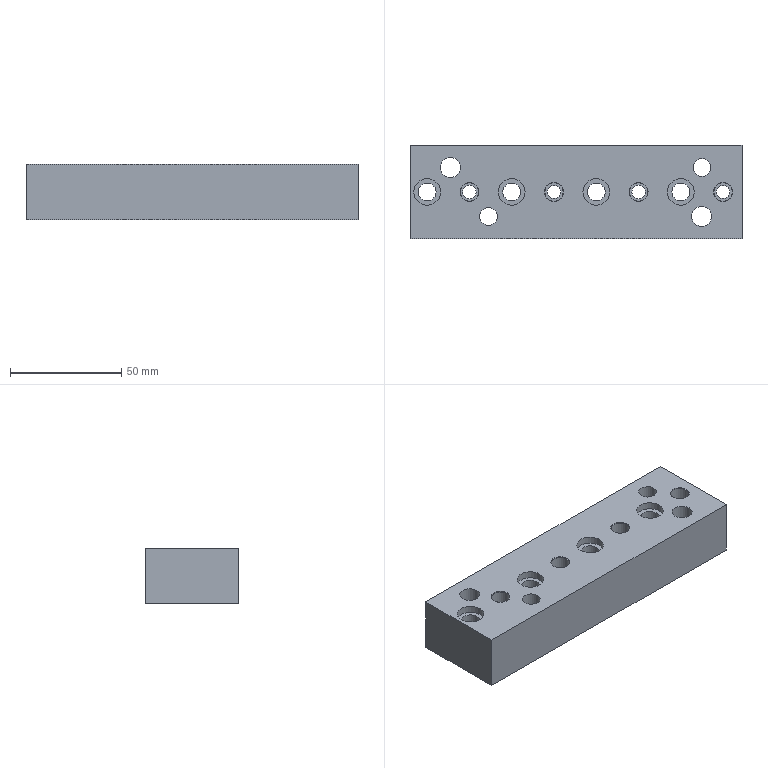Part | STEP file | PN_0036_id230_x_t | 1 solid | 46 faces | box 149.23 x 42 x 25 mm | volume 138214 mm3 | cylinder 26 | plane 20 | commonest cylinder face diameters 8 x6 6 x4 8.2 x4 8.5 x4 12 x4 9 x2
STEP:
#1=CARTESIAN_POINT('',(87.422,21.,25.));
#2=VERTEX_POINT('',#1);
#3=CARTESIAN_POINT('',(236.5,21.,25.));
#4=VERTEX_POINT('',#3);
#5=CARTESIAN_POINT('',(27.5,21.,25.));
#6=DIRECTION('',(1.,0.,0.));
#7=VECTOR('',#6,1.);
#8=LINE('',#5,#7);
#9=EDGE_CURVE('',#2,#4,#8,.T.);
#10=ORIENTED_EDGE('',*,*,#9,.T.);
#11=CARTESIAN_POINT('',(236.5,21.,0.));
#12=VERTEX_POINT('',#11);
#13=CARTESIAN_POINT('',(236.5,21.,12.5));
#14=DIRECTION('',(0.,0.,1.));
#15=VECTOR('',#14,1.);
#16=LINE('',#13,#15);
#17=EDGE_CURVE('',#12,#4,#16,.T.);
#18=ORIENTED_EDGE('',*,*,#17,.F.);
#19=CARTESIAN_POINT('',(87.422,21.,0.));
#20=VERTEX_POINT('',#19);
#21=CARTESIAN_POINT('',(27.5,21.,0.));
#22=DIRECTION('',(-1.,0.,0.));
#23=VECTOR('',#22,1.);
#24=LINE('',#21,#23);
#25=EDGE_CURVE('',#12,#20,#24,.T.);
#26=ORIENTED_EDGE('',*,*,#25,.T.);
#27=CARTESIAN_POINT('',(87.422,21.,12.5));
#28=DIRECTION('',(0.,0.,1.));
#29=VECTOR('',#28,1.);
#30=LINE('',#27,#29);
#31=EDGE_CURVE('',#20,#2,#30,.T.);
#32=ORIENTED_EDGE('',*,*,#31,.T.);
#33=EDGE_LOOP('',(#10,#18,#26,#32));
#34=FACE_OUTER_BOUND('',#33,.T.);
#35=CARTESIAN_POINT('',(47.5,21.,12.5));
#36=DIRECTION('',(0.,1.,0.));
#37=DIRECTION('',(0.,0.,1.));
#38=AXIS2_PLACEMENT_3D('',#35,#36,#37);
#39=PLANE('',#38);
#40=ADVANCED_FACE('',(#34),#39,.T.);
#41=CARTESIAN_POINT('',(87.27,-21.,0.));
#42=VERTEX_POINT('',#41);
#43=CARTESIAN_POINT('',(236.5,-21.,0.));
#44=VERTEX_POINT('',#43);
#45=CARTESIAN_POINT('',(27.5,-21.,0.));
#46=DIRECTION('',(1.,0.,0.));
#47=VECTOR('',#46,1.);
#48=LINE('',#45,#47);
#49=EDGE_CURVE('',#42,#44,#48,.T.);
#50=ORIENTED_EDGE('',*,*,#49,.T.);
#51=CARTESIAN_POINT('',(236.5,-21.,25.));
#52=VERTEX_POINT('',#51);
#53=CARTESIAN_POINT('',(236.5,-21.,12.5));
#54=DIRECTION('',(0.,0.,1.));
#55=VECTOR('',#54,1.);
#56=LINE('',#53,#55);
#57=EDGE_CURVE('',#44,#52,#56,.T.);
#58=ORIENTED_EDGE('',*,*,#57,.T.);
#59=CARTESIAN_POINT('',(87.27,-21.,25.));
#60=VERTEX_POINT('',#59);
#61=CARTESIAN_POINT('',(27.5,-21.,25.));
#62=DIRECTION('',(-1.,0.,0.));
#63=VECTOR('',#62,1.);
#64=LINE('',#61,#63);
#65=EDGE_CURVE('',#52,#60,#64,.T.);
#66=ORIENTED_EDGE('',*,*,#65,.T.);
#67=CARTESIAN_POINT('',(87.27,-21.,25.818));
#68=DIRECTION('',(0.,0.,1.));
#69=VECTOR('',#68,1.);
#70=LINE('',#67,#69);
#71=EDGE_CURVE('',#42,#60,#70,.T.);
#72=ORIENTED_EDGE('',*,*,#71,.F.);
#73=EDGE_LOOP('',(#50,#58,#66,#72));
#74=FACE_OUTER_BOUND('',#73,.T.);
#75=CARTESIAN_POINT('',(110.347,-21.,25.818));
#76=DIRECTION('',(0.,1.,0.));
#77=DIRECTION('',(0.,0.,1.));
#78=AXIS2_PLACEMENT_3D('',#75,#76,#77);
#79=PLANE('',#78);
#80=ADVANCED_FACE('',(#74),#79,.F.);
#81=CARTESIAN_POINT('',(118.5,-11.,25.));
#82=VERTEX_POINT('',#81);
#83=CARTESIAN_POINT('',(122.5,-11.,25.));
#84=DIRECTION('',(0.,0.,-1.));
#85=DIRECTION('',(-1.,0.,0.));
#86=AXIS2_PLACEMENT_3D('',#83,#84,#85);
#87=CIRCLE('',#86,4.);
#88=EDGE_CURVE('',#82,#82,#87,.T.);
#89=ORIENTED_EDGE('',*,*,#88,.T.);
#90=EDGE_LOOP('',(#89));
#91=FACE_BOUND('',#90,.T.);
#92=CARTESIAN_POINT('',(214.5,11.,25.));
#93=VERTEX_POINT('',#92);
#94=CARTESIAN_POINT('',(218.5,11.,25.));
#95=DIRECTION('',(0.,0.,-1.));
#96=DIRECTION('',(-1.,0.,0.));
#97=AXIS2_PLACEMENT_3D('',#94,#95,#96);
#98=CIRCLE('',#97,4.);
#99=EDGE_CURVE('',#93,#93,#98,.T.);
#100=ORIENTED_EDGE('',*,*,#99,.T.);
#101=EDGE_LOOP('',(#100));
#102=FACE_BOUND('',#101,.T.);
#103=CARTESIAN_POINT('',(222.848,-11.,25.));
#104=VERTEX_POINT('',#103);
#105=CARTESIAN_POINT('',(218.348,-11.,25.));
#106=DIRECTION('',(0.,0.,-1.));
#107=DIRECTION('',(1.,0.,0.));
#108=AXIS2_PLACEMENT_3D('',#105,#106,#107);
#109=CIRCLE('',#108,4.5);
#110=EDGE_CURVE('',#104,#104,#109,.T.);
#111=ORIENTED_EDGE('',*,*,#110,.T.);
#112=EDGE_LOOP('',(#111));
#113=FACE_BOUND('',#112,.T.);
#114=CARTESIAN_POINT('',(100.922,11.,25.));
#115=VERTEX_POINT('',#114);
#116=CARTESIAN_POINT('',(105.422,11.,25.));
#117=DIRECTION('',(0.,0.,-1.));
#118=DIRECTION('',(-1.,0.,0.));
#119=AXIS2_PLACEMENT_3D('',#116,#117,#118);
#120=CIRCLE('',#119,4.5);
#121=EDGE_CURVE('',#115,#115,#120,.T.);
#122=ORIENTED_EDGE('',*,*,#121,.T.);
#123=EDGE_LOOP('',(#122));
#124=FACE_BOUND('',#123,.T.);
#125=CARTESIAN_POINT('',(232.25,0.,25.));
#126=VERTEX_POINT('',#125);
#127=CARTESIAN_POINT('',(228.,0.,25.));
#128=DIRECTION('',(0.,0.,1.));
#129=DIRECTION('',(1.,0.,0.));
#130=AXIS2_PLACEMENT_3D('',#127,#128,#129);
#131=CIRCLE('',#130,4.25);
#132=EDGE_CURVE('',#126,#126,#131,.T.);
#133=ORIENTED_EDGE('',*,*,#132,.F.);
#134=EDGE_LOOP('',(#133));
#135=FACE_BOUND('',#134,.T.);
#136=CARTESIAN_POINT('',(194.25,0.,25.));
#137=VERTEX_POINT('',#136);
#138=CARTESIAN_POINT('',(190.,0.,25.));
#139=DIRECTION('',(0.,0.,1.));
#140=DIRECTION('',(1.,0.,0.));
#141=AXIS2_PLACEMENT_3D('',#138,#139,#140);
#142=CIRCLE('',#141,4.25);
#143=EDGE_CURVE('',#137,#137,#142,.T.);
#144=ORIENTED_EDGE('',*,*,#143,.F.);
#145=EDGE_LOOP('',(#144));
#146=FACE_BOUND('',#145,.T.);
#147=CARTESIAN_POINT('',(156.25,0.,25.));
#148=VERTEX_POINT('',#147);
#149=CARTESIAN_POINT('',(152.,0.,25.));
#150=DIRECTION('',(0.,0.,1.));
#151=DIRECTION('',(1.,0.,0.));
#152=AXIS2_PLACEMENT_3D('',#149,#150,#151);
#153=CIRCLE('',#152,4.25);
#154=EDGE_CURVE('',#148,#148,#153,.T.);
#155=ORIENTED_EDGE('',*,*,#154,.F.);
#156=EDGE_LOOP('',(#155));
#157=FACE_BOUND('',#156,.T.);
#158=CARTESIAN_POINT('',(118.25,0.,25.));
#159=VERTEX_POINT('',#158);
#160=CARTESIAN_POINT('',(114.,0.,25.));
#161=DIRECTION('',(0.,0.,1.));
#162=DIRECTION('',(1.,0.,0.));
#163=AXIS2_PLACEMENT_3D('',#160,#161,#162);
#164=CIRCLE('',#163,4.25);
#165=EDGE_CURVE('',#159,#159,#164,.T.);
#166=ORIENTED_EDGE('',*,*,#165,.F.);
#167=EDGE_LOOP('',(#166));
#168=FACE_BOUND('',#167,.T.);
#169=CARTESIAN_POINT('',(215.,0.,25.));
#170=VERTEX_POINT('',#169);
#171=CARTESIAN_POINT('',(209.,0.,25.));
#172=DIRECTION('',(0.,0.,-1.));
#173=DIRECTION('',(1.,0.,0.));
#174=AXIS2_PLACEMENT_3D('',#171,#172,#173);
#175=CIRCLE('',#174,6.);
#176=EDGE_CURVE('',#170,#170,#175,.T.);
#177=ORIENTED_EDGE('',*,*,#176,.T.);
#178=EDGE_LOOP('',(#177));
#179=FACE_BOUND('',#178,.T.);
#180=CARTESIAN_POINT('',(177.,0.,25.));
#181=VERTEX_POINT('',#180);
#182=CARTESIAN_POINT('',(171.,0.,25.));
#183=DIRECTION('',(0.,0.,-1.));
#184=DIRECTION('',(1.,0.,0.));
#185=AXIS2_PLACEMENT_3D('',#182,#183,#184);
#186=CIRCLE('',#185,6.);
#187=EDGE_CURVE('',#181,#181,#186,.T.);
#188=ORIENTED_EDGE('',*,*,#187,.T.);
#189=EDGE_LOOP('',(#188));
#190=FACE_BOUND('',#189,.T.);
#191=CARTESIAN_POINT('',(139.,0.,25.));
#192=VERTEX_POINT('',#191);
#193=CARTESIAN_POINT('',(133.,0.,25.));
#194=DIRECTION('',(0.,0.,-1.));
#195=DIRECTION('',(1.,0.,0.));
#196=AXIS2_PLACEMENT_3D('',#193,#194,#195);
#197=CIRCLE('',#196,6.);
#198=EDGE_CURVE('',#192,#192,#197,.T.);
#199=ORIENTED_EDGE('',*,*,#198,.T.);
#200=EDGE_LOOP('',(#199));
#201=FACE_BOUND('',#200,.T.);
#202=CARTESIAN_POINT('',(101.,0.,25.));
#203=VERTEX_POINT('',#202);
#204=CARTESIAN_POINT('',(95.,0.,25.));
#205=DIRECTION('',(0.,0.,-1.));
#206=DIRECTION('',(1.,0.,0.));
#207=AXIS2_PLACEMENT_3D('',#204,#205,#206);
#208=CIRCLE('',#207,6.);
#209=EDGE_CURVE('',#203,#203,#208,.T.);
#210=ORIENTED_EDGE('',*,*,#209,.T.);
#211=EDGE_LOOP('',(#210));
#212=FACE_BOUND('',#211,.T.);
#213=ORIENTED_EDGE('',*,*,#65,.F.);
#214=CARTESIAN_POINT('',(236.5,-7.4,25.));
#215=DIRECTION('',(0.,-1.,0.));
#216=VECTOR('',#215,1.);
#217=LINE('',#214,#216);
#218=EDGE_CURVE('',#4,#52,#217,.T.);
#219=ORIENTED_EDGE('',*,*,#218,.F.);
#220=ORIENTED_EDGE('',*,*,#9,.F.);
#221=CARTESIAN_POINT('',(87.319,-7.617,25.));
#222=DIRECTION('',(-0.003625,-1.,0.));
#223=VECTOR('',#222,1.);
#224=LINE('',#221,#223);
#225=EDGE_CURVE('',#2,#60,#224,.T.);
#226=ORIENTED_EDGE('',*,*,#225,.T.);
#227=EDGE_LOOP('',(#213,#219,#220,#226));
#228=FACE_BOUND('',#227,.T.);
#229=CARTESIAN_POINT('',(27.5,-7.4,25.));
#230=DIRECTION('',(0.,0.,1.));
#231=DIRECTION('',(0.,-1.,0.));
#232=AXIS2_PLACEMENT_3D('',#229,#230,#231);
#233=PLANE('',#232);
#234=ADVANCED_FACE('',(#91,#102,#113,#124,#135,#146,#157,#168,#179,#190,#201,#212,#228),#233,.T.);
#235=CARTESIAN_POINT('',(118.5,-11.,0.));
#236=VERTEX_POINT('',#235);
#237=CARTESIAN_POINT('',(122.5,-11.,0.));
#238=DIRECTION('',(0.,0.,1.));
#239=DIRECTION('',(-1.,0.,0.));
#240=AXIS2_PLACEMENT_3D('',#237,#238,#239);
#241=CIRCLE('',#240,4.);
#242=EDGE_CURVE('',#236,#236,#241,.T.);
#243=ORIENTED_EDGE('',*,*,#242,.T.);
#244=EDGE_LOOP('',(#243));
#245=FACE_BOUND('',#244,.T.);
#246=CARTESIAN_POINT('',(214.5,11.,0.));
#247=VERTEX_POINT('',#246);
#248=CARTESIAN_POINT('',(218.5,11.,0.));
#249=DIRECTION('',(0.,0.,1.));
#250=DIRECTION('',(-1.,0.,0.));
#251=AXIS2_PLACEMENT_3D('',#248,#249,#250);
#252=CIRCLE('',#251,4.);
#253=EDGE_CURVE('',#247,#247,#252,.T.);
#254=ORIENTED_EDGE('',*,*,#253,.T.);
#255=EDGE_LOOP('',(#254));
#256=FACE_BOUND('',#255,.T.);
#257=CARTESIAN_POINT('',(211.348,-11.,0.));
#258=VERTEX_POINT('',#257);
#259=CARTESIAN_POINT('',(218.348,-11.,0.));
#260=DIRECTION('',(0.,0.,1.));
#261=DIRECTION('',(-1.,0.,0.));
#262=AXIS2_PLACEMENT_3D('',#259,#260,#261);
#263=CIRCLE('',#262,7.);
#264=EDGE_CURVE('',#258,#258,#263,.T.);
#265=ORIENTED_EDGE('',*,*,#264,.T.);
#266=EDGE_LOOP('',(#265));
#267=FACE_BOUND('',#266,.T.);
#268=CARTESIAN_POINT('',(112.422,11.,0.));
#269=VERTEX_POINT('',#268);
#270=CARTESIAN_POINT('',(105.422,11.,0.));
#271=DIRECTION('',(0.,0.,1.));
#272=DIRECTION('',(1.,0.,0.));
#273=AXIS2_PLACEMENT_3D('',#270,#271,#272);
#274=CIRCLE('',#273,7.);
#275=EDGE_CURVE('',#269,#269,#274,.T.);
#276=ORIENTED_EDGE('',*,*,#275,.T.);
#277=EDGE_LOOP('',(#276));
#278=FACE_BOUND('',#277,.T.);
#279=CARTESIAN_POINT('',(231.,0.,0.));
#280=VERTEX_POINT('',#279);
#281=CARTESIAN_POINT('',(228.,0.,0.));
#282=DIRECTION('',(0.,0.,-1.));
#283=DIRECTION('',(1.,0.,0.));
#284=AXIS2_PLACEMENT_3D('',#281,#282,#283);
#285=CIRCLE('',#284,3.);
#286=EDGE_CURVE('',#280,#280,#285,.T.);
#287=ORIENTED_EDGE('',*,*,#286,.F.);
#288=EDGE_LOOP('',(#287));
#289=FACE_BOUND('',#288,.T.);
#290=CARTESIAN_POINT('',(193.,0.,0.));
#291=VERTEX_POINT('',#290);
#292=CARTESIAN_POINT('',(190.,0.,0.));
#293=DIRECTION('',(0.,0.,-1.));
#294=DIRECTION('',(1.,0.,0.));
#295=AXIS2_PLACEMENT_3D('',#292,#293,#294);
#296=CIRCLE('',#295,3.);
#297=EDGE_CURVE('',#291,#291,#296,.T.);
#298=ORIENTED_EDGE('',*,*,#297,.F.);
#299=EDGE_LOOP('',(#298));
#300=FACE_BOUND('',#299,.T.);
#301=CARTESIAN_POINT('',(155.,0.,0.));
#302=VERTEX_POINT('',#301);
#303=CARTESIAN_POINT('',(152.,0.,0.));
#304=DIRECTION('',(0.,0.,-1.));
#305=DIRECTION('',(1.,0.,0.));
#306=AXIS2_PLACEMENT_3D('',#303,#304,#305);
#307=CIRCLE('',#306,3.);
#308=EDGE_CURVE('',#302,#302,#307,.T.);
#309=ORIENTED_EDGE('',*,*,#308,.F.);
#310=EDGE_LOOP('',(#309));
#311=FACE_BOUND('',#310,.T.);
#312=CARTESIAN_POINT('',(117.,0.,0.));
#313=VERTEX_POINT('',#312);
#314=CARTESIAN_POINT('',(114.,0.,0.));
#315=DIRECTION('',(0.,0.,-1.));
#316=DIRECTION('',(1.,0.,0.));
#317=AXIS2_PLACEMENT_3D('',#314,#315,#316);
#318=CIRCLE('',#317,3.);
#319=EDGE_CURVE('',#313,#313,#318,.T.);
#320=ORIENTED_EDGE('',*,*,#319,.F.);
#321=EDGE_LOOP('',(#320));
#322=FACE_BOUND('',#321,.T.);
#323=CARTESIAN_POINT('',(213.,0.,0.));
#324=VERTEX_POINT('',#323);
#325=CARTESIAN_POINT('',(209.,0.,0.));
#326=DIRECTION('',(0.,0.,1.));
#327=DIRECTION('',(1.,0.,0.));
#328=AXIS2_PLACEMENT_3D('',#325,#326,#327);
#329=CIRCLE('',#328,4.);
#330=EDGE_CURVE('',#324,#324,#329,.T.);
#331=ORIENTED_EDGE('',*,*,#330,.T.);
#332=EDGE_LOOP('',(#331));
#333=FACE_BOUND('',#332,.T.);
#334=CARTESIAN_POINT('',(175.,0.,0.));
#335=VERTEX_POINT('',#334);
#336=CARTESIAN_POINT('',(171.,0.,0.));
#337=DIRECTION('',(0.,0.,1.));
#338=DIRECTION('',(1.,0.,0.));
#339=AXIS2_PLACEMENT_3D('',#336,#337,#338);
#340=CIRCLE('',#339,4.);
#341=EDGE_CURVE('',#335,#335,#340,.T.);
#342=ORIENTED_EDGE('',*,*,#341,.T.);
#343=EDGE_LOOP('',(#342));
#344=FACE_BOUND('',#343,.T.);
#345=CARTESIAN_POINT('',(137.,0.,0.));
#346=VERTEX_POINT('',#345);
#347=CARTESIAN_POINT('',(133.,0.,0.));
#348=DIRECTION('',(0.,0.,1.));
#349=DIRECTION('',(1.,0.,0.));
#350=AXIS2_PLACEMENT_3D('',#347,#348,#349);
#351=CIRCLE('',#350,4.);
#352=EDGE_CURVE('',#346,#346,#351,.T.);
#353=ORIENTED_EDGE('',*,*,#352,.T.);
#354=EDGE_LOOP('',(#353));
#355=FACE_BOUND('',#354,.T.);
#356=CARTESIAN_POINT('',(99.,0.,0.));
#357=VERTEX_POINT('',#356);
#358=CARTESIAN_POINT('',(95.,0.,0.));
#359=DIRECTION('',(0.,0.,1.));
#360=DIRECTION('',(1.,0.,0.));
#361=AXIS2_PLACEMENT_3D('',#358,#359,#360);
#362=CIRCLE('',#361,4.);
#363=EDGE_CURVE('',#357,#357,#362,.T.);
#364=ORIENTED_EDGE('',*,*,#363,.T.);
#365=EDGE_LOOP('',(#364));
#366=FACE_BOUND('',#365,.T.);
#367=ORIENTED_EDGE('',*,*,#25,.F.);
#368=CARTESIAN_POINT('',(236.5,61.,0.));
#369=DIRECTION('',(0.,1.,0.));
#370=VECTOR('',#369,1.);
#371=LINE('',#368,#370);
#372=EDGE_CURVE('',#44,#12,#371,.T.);
#373=ORIENTED_EDGE('',*,*,#372,.F.);
#374=ORIENTED_EDGE('',*,*,#49,.F.);
#375=CARTESIAN_POINT('',(87.268,-21.505,0.));
#376=DIRECTION('',(-0.003625,-1.,0.));
#377=VECTOR('',#376,1.);
#378=LINE('',#375,#377);
#379=EDGE_CURVE('',#20,#42,#378,.T.);
#380=ORIENTED_EDGE('',*,*,#379,.F.);
#381=EDGE_LOOP('',(#367,#373,#374,#380));
#382=FACE_BOUND('',#381,.T.);
#383=CARTESIAN_POINT('',(27.5,-7.4,0.));
#384=DIRECTION('',(0.,0.,1.));
#385=DIRECTION('',(0.,-1.,0.));
#386=AXIS2_PLACEMENT_3D('',#383,#384,#385);
#387=PLANE('',#386);
#388=ADVANCED_FACE('',(#245,#256,#267,#278,#289,#300,#311,#322,#333,#344,#355,#366,#382),#387,.F.);
#389=ORIENTED_EDGE('',*,*,#379,.T.);
#390=ORIENTED_EDGE('',*,*,#71,.T.);
#391=ORIENTED_EDGE('',*,*,#225,.F.);
#392=ORIENTED_EDGE('',*,*,#31,.F.);
#393=EDGE_LOOP('',(#389,#390,#391,#392));
#394=FACE_OUTER_BOUND('',#393,.T.);
#395=CARTESIAN_POINT('',(87.268,-21.505,-51.));
#396=DIRECTION('',(-1.,0.003625,0.));
#397=DIRECTION('',(-0.003625,-1.,0.));
#398=AXIS2_PLACEMENT_3D('',#395,#396,#397);
#399=PLANE('',#398);
#400=ADVANCED_FACE('',(#394),#399,.T.);
#401=ORIENTED_EDGE('',*,*,#57,.F.);
#402=ORIENTED_EDGE('',*,*,#372,.T.);
#403=ORIENTED_EDGE('',*,*,#17,.T.);
#404=ORIENTED_EDGE('',*,*,#218,.T.);
#405=EDGE_LOOP('',(#401,#402,#403,#404));
#406=FACE_OUTER_BOUND('',#405,.T.);
#407=CARTESIAN_POINT('',(236.5,61.,12.5));
#408=DIRECTION('',(-1.,0.,0.));
#409=DIRECTION('',(0.,0.,1.));
#410=AXIS2_PLACEMENT_3D('',#407,#408,#409);
#411=PLANE('',#410);
#412=ADVANCED_FACE('',(#406),#411,.F.);
#413=CARTESIAN_POINT('',(91.,0.,21.7));
#414=VERTEX_POINT('',#413);
#415=CARTESIAN_POINT('',(95.,0.,21.7));
#416=DIRECTION('',(0.,0.,-1.));
#417=DIRECTION('',(-1.,0.,0.));
#418=AXIS2_PLACEMENT_3D('',#415,#416,#417);
#419=CIRCLE('',#418,4.);
#420=EDGE_CURVE('',#414,#414,#419,.T.);
#421=ORIENTED_EDGE('',*,*,#420,.F.);
#422=EDGE_LOOP('',(#421));
#423=FACE_BOUND('',#422,.T.);
#424=ORIENTED_EDGE('',*,*,#363,.F.);
#425=EDGE_LOOP('',(#424));
#426=FACE_BOUND('',#425,.T.);
#427=CARTESIAN_POINT('',(95.,0.,9.95));
#428=DIRECTION('',(0.,0.,-1.));
#429=DIRECTION('',(-0.008727,1.,0.));
#430=AXIS2_PLACEMENT_3D('',#427,#428,#429);
#431=CYLINDRICAL_SURFACE('',#430,4.);
#432=ADVANCED_FACE('',(#423,#426),#431,.F.);
#433=ORIENTED_EDGE('',*,*,#420,.T.);
#434=EDGE_LOOP('',(#433));
#435=FACE_BOUND('',#434,.T.);
#436=CARTESIAN_POINT('',(89.,0.,21.7));
#437=VERTEX_POINT('',#436);
#438=CARTESIAN_POINT('',(95.,0.,21.7));
#439=DIRECTION('',(0.,0.,-1.));
#440=DIRECTION('',(-1.,0.,0.));
#441=AXIS2_PLACEMENT_3D('',#438,#439,#440);
#442=CIRCLE('',#441,6.);
#443=EDGE_CURVE('',#437,#437,#442,.T.);
#444=ORIENTED_EDGE('',*,*,#443,.F.);
#445=EDGE_LOOP('',(#444));
#446=FACE_BOUND('',#445,.T.);
#447=CARTESIAN_POINT('',(95.,0.,21.7));
#448=DIRECTION('',(0.,0.,-1.));
#449=DIRECTION('',(-1.,0.,0.));
#450=AXIS2_PLACEMENT_3D('',#447,#448,#449);
#451=PLANE('',#450);
#452=ADVANCED_FACE('',(#435,#446),#451,.F.);
#453=ORIENTED_EDGE('',*,*,#443,.T.);
#454=EDGE_LOOP('',(#453));
#455=FACE_BOUND('',#454,.T.);
#456=ORIENTED_EDGE('',*,*,#209,.F.);
#457=EDGE_LOOP('',(#456));
#458=FACE_BOUND('',#457,.T.);
#459=CARTESIAN_POINT('',(95.,0.,23.2));
#460=DIRECTION('',(0.,0.,-1.));
#461=DIRECTION('',(-1.,0.,0.));
#462=AXIS2_PLACEMENT_3D('',#459,#460,#461);
#463=CYLINDRICAL_SURFACE('',#462,6.);
#464=ADVANCED_FACE('',(#455,#458),#463,.F.);
#465=CARTESIAN_POINT('',(129.,0.,21.7));
#466=VERTEX_POINT('',#465);
#467=CARTESIAN_POINT('',(133.,0.,21.7));
#468=DIRECTION('',(0.,0.,-1.));
#469=DIRECTION('',(-1.,0.,0.));
#470=AXIS2_PLACEMENT_3D('',#467,#468,#469);
#471=CIRCLE('',#470,4.);
#472=EDGE_CURVE('',#466,#466,#471,.T.);
#473=ORIENTED_EDGE('',*,*,#472,.F.);
#474=EDGE_LOOP('',(#473));
#475=FACE_BOUND('',#474,.T.);
#476=ORIENTED_EDGE('',*,*,#352,.F.);
#477=EDGE_LOOP('',(#476));
#478=FACE_BOUND('',#477,.T.);
#479=CARTESIAN_POINT('',(133.,0.,9.95));
#480=DIRECTION('',(0.,0.,-1.));
#481=DIRECTION('',(-0.008727,1.,0.));
#482=AXIS2_PLACEMENT_3D('',#479,#480,#481);
#483=CYLINDRICAL_SURFACE('',#482,4.);
#484=ADVANCED_FACE('',(#475,#478),#483,.F.);
#485=ORIENTED_EDGE('',*,*,#472,.T.);
#486=EDGE_LOOP('',(#485));
#487=FACE_BOUND('',#486,.T.);
#488=CARTESIAN_POINT('',(127.,0.,21.7));
#489=VERTEX_POINT('',#488);
#490=CARTESIAN_POINT('',(133.,0.,21.7));
#491=DIRECTION('',(0.,0.,-1.));
#492=DIRECTION('',(-1.,0.,0.));
#493=AXIS2_PLACEMENT_3D('',#490,#491,#492);
#494=CIRCLE('',#493,6.);
#495=EDGE_CURVE('',#489,#489,#494,.T.);
#496=ORIENTED_EDGE('',*,*,#495,.F.);
#497=EDGE_LOOP('',(#496));
#498=FACE_BOUND('',#497,.T.);
#499=CARTESIAN_POINT('',(133.,0.,21.7));
#500=DIRECTION('',(0.,0.,-1.));
#501=DIRECTION('',(-1.,0.,0.));
#502=AXIS2_PLACEMENT_3D('',#499,#500,#501);
#503=PLANE('',#502);
#504=ADVANCED_FACE('',(#487,#498),#503,.F.);
#505=ORIENTED_EDGE('',*,*,#495,.T.);
#506=EDGE_LOOP('',(#505));
#507=FACE_BOUND('',#506,.T.);
#508=ORIENTED_EDGE('',*,*,#198,.F.);
#509=EDGE_LOOP('',(#508));
#510=FACE_BOUND('',#509,.T.);
#511=CARTESIAN_POINT('',(133.,0.,23.2));
#512=DIRECTION('',(0.,0.,-1.));
#513=DIRECTION('',(-1.,0.,0.));
#514=AXIS2_PLACEMENT_3D('',#511,#512,#513);
#515=CYLINDRICAL_SURFACE('',#514,6.);
#516=ADVANCED_FACE('',(#507,#510),#515,.F.);
#517=CARTESIAN_POINT('',(167.,0.,21.7));
#518=VERTEX_POINT('',#517);
#519=CARTESIAN_POINT('',(171.,0.,21.7));
#520=DIRECTION('',(0.,0.,-1.));
#521=DIRECTION('',(-1.,0.,0.));
#522=AXIS2_PLACEMENT_3D('',#519,#520,#521);
#523=CIRCLE('',#522,4.);
#524=EDGE_CURVE('',#518,#518,#523,.T.);
#525=ORIENTED_EDGE('',*,*,#524,.F.);
#526=EDGE_LOOP('',(#525));
#527=FACE_BOUND('',#526,.T.);
#528=ORIENTED_EDGE('',*,*,#341,.F.);
#529=EDGE_LOOP('',(#528));
#530=FACE_BOUND('',#529,.T.);
#531=CARTESIAN_POINT('',(171.,0.,9.95));
#532=DIRECTION('',(0.,0.,-1.));
#533=DIRECTION('',(-0.008727,1.,0.));
#534=AXIS2_PLACEMENT_3D('',#531,#532,#533);
#535=CYLINDRICAL_SURFACE('',#534,4.);
#536=ADVANCED_FACE('',(#527,#530),#535,.F.);
#537=ORIENTED_EDGE('',*,*,#524,.T.);
#538=EDGE_LOOP('',(#537));
#539=FACE_BOUND('',#538,.T.);
#540=CARTESIAN_POINT('',(165.,0.,21.7));
#541=VERTEX_POINT('',#540);
#542=CARTESIAN_POINT('',(171.,0.,21.7));
#543=DIRECTION('',(0.,0.,-1.));
#544=DIRECTION('',(-1.,0.,0.));
#545=AXIS2_PLACEMENT_3D('',#542,#543,#544);
#546=CIRCLE('',#545,6.);
#547=EDGE_CURVE('',#541,#541,#546,.T.);
#548=ORIENTED_EDGE('',*,*,#547,.F.);
#549=EDGE_LOOP('',(#548));
#550=FACE_BOUND('',#549,.T.);
#551=CARTESIAN_POINT('',(171.,0.,21.7));
#552=DIRECTION('',(0.,0.,-1.));
#553=DIRECTION('',(-1.,0.,0.));
#554=AXIS2_PLACEMENT_3D('',#551,#552,#553);
#555=PLANE('',#554);
#556=ADVANCED_FACE('',(#539,#550),#555,.F.);
#557=ORIENTED_EDGE('',*,*,#547,.T.);
#558=EDGE_LOOP('',(#557));
#559=FACE_BOUND('',#558,.T.);
#560=ORIENTED_EDGE('',*,*,#187,.F.);
#561=EDGE_LOOP('',(#560));
#562=FACE_BOUND('',#561,.T.);
#563=CARTESIAN_POINT('',(171.,0.,23.2));
#564=DIRECTION('',(0.,0.,-1.));
#565=DIRECTION('',(-1.,0.,0.));
#566=AXIS2_PLACEMENT_3D('',#563,#564,#565);
#567=CYLINDRICAL_SURFACE('',#566,6.);
#568=ADVANCED_FACE('',(#559,#562),#567,.F.);
#569=CARTESIAN_POINT('',(205.,0.,21.7));
#570=VERTEX_POINT('',#569);
#571=CARTESIAN_POINT('',(209.,0.,21.7));
#572=DIRECTION('',(0.,0.,-1.));
#573=DIRECTION('',(-1.,0.,0.));
#574=AXIS2_PLACEMENT_3D('',#571,#572,#573);
#575=CIRCLE('',#574,4.);
#576=EDGE_CURVE('',#570,#570,#575,.T.);
#577=ORIENTED_EDGE('',*,*,#576,.F.);
#578=EDGE_LOOP('',(#577));
#579=FACE_BOUND('',#578,.T.);
#580=ORIENTED_EDGE('',*,*,#330,.F.);
#581=EDGE_LOOP('',(#580));
#582=FACE_BOUND('',#581,.T.);
#583=CARTESIAN_POINT('',(209.,0.,9.95));
#584=DIRECTION('',(0.,0.,-1.));
#585=DIRECTION('',(-0.008727,1.,0.));
#586=AXIS2_PLACEMENT_3D('',#583,#584,#585);
#587=CYLINDRICAL_SURFACE('',#586,4.);
#588=ADVANCED_FACE('',(#579,#582),#587,.F.);
#589=ORIENTED_EDGE('',*,*,#576,.T.);
#590=EDGE_LOOP('',(#589));
#591=FACE_BOUND('',#590,.T.);
#592=CARTESIAN_POINT('',(203.,0.,21.7));
#593=VERTEX_POINT('',#592);
#594=CARTESIAN_POINT('',(209.,0.,21.7));
#595=DIRECTION('',(0.,0.,-1.));
#596=DIRECTION('',(-1.,0.,0.));
#597=AXIS2_PLACEMENT_3D('',#594,#595,#596);
#598=CIRCLE('',#597,6.);
#599=EDGE_CURVE('',#593,#593,#598,.T.);
#600=ORIENTED_EDGE('',*,*,#599,.F.);
#601=EDGE_LOOP('',(#600));
#602=FACE_BOUND('',#601,.T.);
#603=CARTESIAN_POINT('',(209.,0.,21.7));
#604=DIRECTION('',(0.,0.,-1.));
#605=DIRECTION('',(-1.,0.,0.));
#606=AXIS2_PLACEMENT_3D('',#603,#604,#605);
#607=PLANE('',#606);
#608=ADVANCED_FACE('',(#591,#602),#607,.F.);
#609=ORIENTED_EDGE('',*,*,#599,.T.);
#610=EDGE_LOOP('',(#609));
#611=FACE_BOUND('',#610,.T.);
#612=ORIENTED_EDGE('',*,*,#176,.F.);
#613=EDGE_LOOP('',(#612));
#614=FACE_BOUND('',#613,.T.);
#615=CARTESIAN_POINT('',(209.,0.,23.2));
#616=DIRECTION('',(0.,0.,-1.));
#617=DIRECTION('',(-1.,0.,0.));
#618=AXIS2_PLACEMENT_3D('',#615,#616,#617);
#619=CYLINDRICAL_SURFACE('',#618,6.);
#620=ADVANCED_FACE('',(#611,#614),#619,.F.);
#621=CARTESIAN_POINT('',(117.,0.,11.7));
#622=VERTEX_POINT('',#621);
#623=CARTESIAN_POINT('',(114.,0.,11.7));
#624=DIRECTION('',(0.,0.,1.));
#625=DIRECTION('',(1.,0.,0.));
#626=AXIS2_PLACEMENT_3D('',#623,#624,#625);
#627=CIRCLE('',#626,3.);
#628=EDGE_CURVE('',#622,#622,#627,.T.);
#629=ORIENTED_EDGE('',*,*,#628,.F.);
#630=EDGE_LOOP('',(#629));
#631=FACE_BOUND('',#630,.T.);
#632=CARTESIAN_POINT('',(118.1,0.,11.7));
#633=VERTEX_POINT('',#632);
#634=CARTESIAN_POINT('',(114.,0.,11.7));
#635=DIRECTION('',(0.,0.,-1.));
#636=DIRECTION('',(1.,0.,0.));
#637=AXIS2_PLACEMENT_3D('',#634,#635,#636);
#638=CIRCLE('',#637,4.1);
#639=EDGE_CURVE('',#633,#633,#638,.T.);
#640=ORIENTED_EDGE('',*,*,#639,.F.);
#641=EDGE_LOOP('',(#640));
#642=FACE_BOUND('',#641,.T.);
#643=CARTESIAN_POINT('',(114.,0.,11.7));
#644=DIRECTION('',(0.,0.,-1.));
#645=DIRECTION('',(1.,0.,0.));
#646=AXIS2_PLACEMENT_3D('',#643,#644,#645);
#647=PLANE('',#646);
#648=ADVANCED_FACE('',(#631,#642),#647,.F.);
#649=CARTESIAN_POINT('',(109.9,0.,24.7));
#650=VERTEX_POINT('',#649);
#651=CARTESIAN_POINT('',(114.,0.,24.7));
#652=DIRECTION('',(0.,0.,1.));
#653=DIRECTION('',(-1.,0.,0.));
#654=AXIS2_PLACEMENT_3D('',#651,#652,#653);
#655=CIRCLE('',#654,4.1);
#656=EDGE_CURVE('',#650,#650,#655,.T.);
#657=ORIENTED_EDGE('',*,*,#656,.T.);
#658=EDGE_LOOP('',(#657));
#659=FACE_BOUND('',#658,.T.);
#660=ORIENTED_EDGE('',*,*,#639,.T.);
#661=EDGE_LOOP('',(#660));
#662=FACE_BOUND('',#661,.T.);
#663=CARTESIAN_POINT('',(114.,0.,11.7));
#664=DIRECTION('',(0.,0.,1.));
#665=DIRECTION('',(1.,0.,0.));
#666=AXIS2_PLACEMENT_3D('',#663,#664,#665);
#667=CYLINDRICAL_SURFACE('',#666,4.1);
#668=ADVANCED_FACE('',(#659,#662),#667,.F.);
#669=ORIENTED_EDGE('',*,*,#319,.T.);
#670=EDGE_LOOP('',(#669));
#671=FACE_BOUND('',#670,.T.);
#672=ORIENTED_EDGE('',*,*,#628,.T.);
#673=EDGE_LOOP('',(#672));
#674=FACE_BOUND('',#673,.T.);
#675=CARTESIAN_POINT('',(114.,0.,11.7));
#676=DIRECTION('',(0.,0.,-1.));
#677=DIRECTION('',(1.,0.,0.));
#678=AXIS2_PLACEMENT_3D('',#675,#676,#677);
#679=CYLINDRICAL_SURFACE('',#678,3.);
#680=ADVANCED_FACE('',(#671,#674),#679,.F.);
#681=CARTESIAN_POINT('',(109.75,0.,24.7));
#682=VERTEX_POINT('',#681);
#683=CARTESIAN_POINT('',(114.,0.,24.7));
#684=DIRECTION('',(0.,0.,-1.));
#685=DIRECTION('',(-1.,0.,0.));
#686=AXIS2_PLACEMENT_3D('',#683,#684,#685);
#687=CIRCLE('',#686,4.25);
#688=EDGE_CURVE('',#682,#682,#687,.T.);
#689=ORIENTED_EDGE('',*,*,#688,.F.);
#690=EDGE_LOOP('',(#689));
#691=FACE_BOUND('',#690,.T.);
#692=ORIENTED_EDGE('',*,*,#656,.F.);
#693=EDGE_LOOP('',(#692));
#694=FACE_BOUND('',#693,.T.);
#695=CARTESIAN_POINT('',(3.225,94.25,24.7));
#696=DIRECTION('',(0.,0.,1.));
#697=DIRECTION('',(-1.,0.,0.));
#698=AXIS2_PLACEMENT_3D('',#695,#696,#697);
#699=PLANE('',#698);
#700=ADVANCED_FACE('',(#691,#694),#699,.T.);
#701=ORIENTED_EDGE('',*,*,#165,.T.);
#702=EDGE_LOOP('',(#701));
#703=FACE_BOUND('',#702,.T.);
#704=ORIENTED_EDGE('',*,*,#688,.T.);
#705=EDGE_LOOP('',(#704));
#706=FACE_BOUND('',#705,.T.);
#707=CARTESIAN_POINT('',(114.,0.,46.7));
#708=DIRECTION('',(0.,0.,1.));
#709=DIRECTION('',(1.,0.,0.));
#710=AXIS2_PLACEMENT_3D('',#707,#708,#709);
#711=CYLINDRICAL_SURFACE('',#710,4.25);
#712=ADVANCED_FACE('',(#703,#706),#711,.F.);
#713=CARTESIAN_POINT('',(155.,0.,11.7));
#714=VERTEX_POINT('',#713);
#715=CARTESIAN_POINT('',(152.,0.,11.7));
#716=DIRECTION('',(0.,0.,1.));
#717=DIRECTION('',(1.,0.,0.));
#718=AXIS2_PLACEMENT_3D('',#715,#716,#717);
#719=CIRCLE('',#718,3.);
#720=EDGE_CURVE('',#714,#714,#719,.T.);
#721=ORIENTED_EDGE('',*,*,#720,.F.);
#722=EDGE_LOOP('',(#721));
#723=FACE_BOUND('',#722,.T.);
#724=CARTESIAN_POINT('',(156.1,0.,11.7));
#725=VERTEX_POINT('',#724);
#726=CARTESIAN_POINT('',(152.,0.,11.7));
#727=DIRECTION('',(0.,0.,-1.));
#728=DIRECTION('',(1.,0.,0.));
#729=AXIS2_PLACEMENT_3D('',#726,#727,#728);
#730=CIRCLE('',#729,4.1);
#731=EDGE_CURVE('',#725,#725,#730,.T.);
#732=ORIENTED_EDGE('',*,*,#731,.F.);
#733=EDGE_LOOP('',(#732));
#734=FACE_BOUND('',#733,.T.);
#735=CARTESIAN_POINT('',(152.,0.,11.7));
#736=DIRECTION('',(0.,0.,-1.));
#737=DIRECTION('',(1.,0.,0.));
#738=AXIS2_PLACEMENT_3D('',#735,#736,#737);
#739=PLANE('',#738);
#740=ADVANCED_FACE('',(#723,#734),#739,.F.);
#741=CARTESIAN_POINT('',(147.9,0.,24.7));
#742=VERTEX_POINT('',#741);
#743=CARTESIAN_POINT('',(152.,0.,24.7));
#744=DIRECTION('',(0.,0.,1.));
#745=DIRECTION('',(-1.,0.,0.));
#746=AXIS2_PLACEMENT_3D('',#743,#744,#745);
#747=CIRCLE('',#746,4.1);
#748=EDGE_CURVE('',#742,#742,#747,.T.);
#749=ORIENTED_EDGE('',*,*,#748,.T.);
#750=EDGE_LOOP('',(#749));
#751=FACE_BOUND('',#750,.T.);
#752=ORIENTED_EDGE('',*,*,#731,.T.);
#753=EDGE_LOOP('',(#752));
#754=FACE_BOUND('',#753,.T.);
#755=CARTESIAN_POINT('',(152.,0.,11.7));
#756=DIRECTION('',(0.,0.,1.));
#757=DIRECTION('',(1.,0.,0.));
#758=AXIS2_PLACEMENT_3D('',#755,#756,#757);
#759=CYLINDRICAL_SURFACE('',#758,4.1);
#760=ADVANCED_FACE('',(#751,#754),#759,.F.);
#761=ORIENTED_EDGE('',*,*,#308,.T.);
#762=EDGE_LOOP('',(#761));
#763=FACE_BOUND('',#762,.T.);
#764=ORIENTED_EDGE('',*,*,#720,.T.);
#765=EDGE_LOOP('',(#764));
#766=FACE_BOUND('',#765,.T.);
#767=CARTESIAN_POINT('',(152.,0.,11.7));
#768=DIRECTION('',(0.,0.,-1.));
#769=DIRECTION('',(1.,0.,0.));
#770=AXIS2_PLACEMENT_3D('',#767,#768,#769);
#771=CYLINDRICAL_SURFACE('',#770,3.);
#772=ADVANCED_FACE('',(#763,#766),#771,.F.);
#773=CARTESIAN_POINT('',(147.75,0.,24.7));
#774=VERTEX_POINT('',#773);
#775=CARTESIAN_POINT('',(152.,0.,24.7));
#776=DIRECTION('',(0.,0.,-1.));
#777=DIRECTION('',(-1.,0.,0.));
#778=AXIS2_PLACEMENT_3D('',#775,#776,#777);
#779=CIRCLE('',#778,4.25);
#780=EDGE_CURVE('',#774,#774,#779,.T.);
#781=ORIENTED_EDGE('',*,*,#780,.F.);
#782=EDGE_LOOP('',(#781));
#783=FACE_BOUND('',#782,.T.);
#784=ORIENTED_EDGE('',*,*,#748,.F.);
#785=EDGE_LOOP('',(#784));
#786=FACE_BOUND('',#785,.T.);
#787=CARTESIAN_POINT('',(41.225,94.25,24.7));
#788=DIRECTION('',(0.,0.,1.));
#789=DIRECTION('',(-1.,0.,0.));
#790=AXIS2_PLACEMENT_3D('',#787,#788,#789);
#791=PLANE('',#790);
#792=ADVANCED_FACE('',(#783,#786),#791,.T.);
#793=ORIENTED_EDGE('',*,*,#154,.T.);
#794=EDGE_LOOP('',(#793));
#795=FACE_BOUND('',#794,.T.);
#796=ORIENTED_EDGE('',*,*,#780,.T.);
#797=EDGE_LOOP('',(#796));
#798=FACE_BOUND('',#797,.T.);
#799=CARTESIAN_POINT('',(152.,0.,46.7));
#800=DIRECTION('',(0.,0.,1.));
#801=DIRECTION('',(1.,0.,0.));
#802=AXIS2_PLACEMENT_3D('',#799,#800,#801);
#803=CYLINDRICAL_SURFACE('',#802,4.25);
#804=ADVANCED_FACE('',(#795,#798),#803,.F.);
#805=CARTESIAN_POINT('',(193.,0.,11.7));
#806=VERTEX_POINT('',#805);
#807=CARTESIAN_POINT('',(190.,0.,11.7));
#808=DIRECTION('',(0.,0.,1.));
#809=DIRECTION('',(1.,0.,0.));
#810=AXIS2_PLACEMENT_3D('',#807,#808,#809);
#811=CIRCLE('',#810,3.);
#812=EDGE_CURVE('',#806,#806,#811,.T.);
#813=ORIENTED_EDGE('',*,*,#812,.F.);
#814=EDGE_LOOP('',(#813));
#815=FACE_BOUND('',#814,.T.);
#816=CARTESIAN_POINT('',(194.1,0.,11.7));
#817=VERTEX_POINT('',#816);
#818=CARTESIAN_POINT('',(190.,0.,11.7));
#819=DIRECTION('',(0.,0.,-1.));
#820=DIRECTION('',(1.,0.,0.));
#821=AXIS2_PLACEMENT_3D('',#818,#819,#820);
#822=CIRCLE('',#821,4.1);
#823=EDGE_CURVE('',#817,#817,#822,.T.);
#824=ORIENTED_EDGE('',*,*,#823,.F.);
#825=EDGE_LOOP('',(#824));
#826=FACE_BOUND('',#825,.T.);
#827=CARTESIAN_POINT('',(190.,0.,11.7));
#828=DIRECTION('',(0.,0.,-1.));
#829=DIRECTION('',(1.,0.,0.));
#830=AXIS2_PLACEMENT_3D('',#827,#828,#829);
#831=PLANE('',#830);
#832=ADVANCED_FACE('',(#815,#826),#831,.F.);
#833=CARTESIAN_POINT('',(185.9,0.,24.7));
#834=VERTEX_POINT('',#833);
#835=CARTESIAN_POINT('',(190.,0.,24.7));
#836=DIRECTION('',(0.,0.,1.));
#837=DIRECTION('',(-1.,0.,0.));
#838=AXIS2_PLACEMENT_3D('',#835,#836,#837);
#839=CIRCLE('',#838,4.1);
#840=EDGE_CURVE('',#834,#834,#839,.T.);
#841=ORIENTED_EDGE('',*,*,#840,.T.);
#842=EDGE_LOOP('',(#841));
#843=FACE_BOUND('',#842,.T.);
#844=ORIENTED_EDGE('',*,*,#823,.T.);
#845=EDGE_LOOP('',(#844));
#846=FACE_BOUND('',#845,.T.);
#847=CARTESIAN_POINT('',(190.,0.,11.7));
#848=DIRECTION('',(0.,0.,1.));
#849=DIRECTION('',(1.,0.,0.));
#850=AXIS2_PLACEMENT_3D('',#847,#848,#849);
#851=CYLINDRICAL_SURFACE('',#850,4.1);
#852=ADVANCED_FACE('',(#843,#846),#851,.F.);
#853=ORIENTED_EDGE('',*,*,#297,.T.);
#854=EDGE_LOOP('',(#853));
#855=FACE_BOUND('',#854,.T.);
#856=ORIENTED_EDGE('',*,*,#812,.T.);
#857=EDGE_LOOP('',(#856));
#858=FACE_BOUND('',#857,.T.);
#859=CARTESIAN_POINT('',(190.,0.,11.7));
#860=DIRECTION('',(0.,0.,-1.));
#861=DIRECTION('',(1.,0.,0.));
#862=AXIS2_PLACEMENT_3D('',#859,#860,#861);
#863=CYLINDRICAL_SURFACE('',#862,3.);
#864=ADVANCED_FACE('',(#855,#858),#863,.F.);
#865=CARTESIAN_POINT('',(185.75,0.,24.7));
#866=VERTEX_POINT('',#865);
#867=CARTESIAN_POINT('',(190.,0.,24.7));
#868=DIRECTION('',(0.,0.,-1.));
#869=DIRECTION('',(-1.,0.,0.));
#870=AXIS2_PLACEMENT_3D('',#867,#868,#869);
#871=CIRCLE('',#870,4.25);
#872=EDGE_CURVE('',#866,#866,#871,.T.);
#873=ORIENTED_EDGE('',*,*,#872,.F.);
#874=EDGE_LOOP('',(#873));
#875=FACE_BOUND('',#874,.T.);
#876=ORIENTED_EDGE('',*,*,#840,.F.);
#877=EDGE_LOOP('',(#876));
#878=FACE_BOUND('',#877,.T.);
#879=CARTESIAN_POINT('',(79.225,94.25,24.7));
#880=DIRECTION('',(0.,0.,1.));
#881=DIRECTION('',(-1.,0.,0.));
#882=AXIS2_PLACEMENT_3D('',#879,#880,#881);
#883=PLANE('',#882);
#884=ADVANCED_FACE('',(#875,#878),#883,.T.);
#885=ORIENTED_EDGE('',*,*,#143,.T.);
#886=EDGE_LOOP('',(#885));
#887=FACE_BOUND('',#886,.T.);
#888=ORIENTED_EDGE('',*,*,#872,.T.);
#889=EDGE_LOOP('',(#888));
#890=FACE_BOUND('',#889,.T.);
#891=CARTESIAN_POINT('',(190.,0.,46.7));
#892=DIRECTION('',(0.,0.,1.));
#893=DIRECTION('',(1.,0.,0.));
#894=AXIS2_PLACEMENT_3D('',#891,#892,#893);
#895=CYLINDRICAL_SURFACE('',#894,4.25);
#896=ADVANCED_FACE('',(#887,#890),#895,.F.);
#897=CARTESIAN_POINT('',(231.,0.,11.7));
#898=VERTEX_POINT('',#897);
#899=CARTESIAN_POINT('',(228.,0.,11.7));
#900=DIRECTION('',(0.,0.,1.));
#901=DIRECTION('',(1.,0.,0.));
#902=AXIS2_PLACEMENT_3D('',#899,#900,#901);
#903=CIRCLE('',#902,3.);
#904=EDGE_CURVE('',#898,#898,#903,.T.);
#905=ORIENTED_EDGE('',*,*,#904,.F.);
#906=EDGE_LOOP('',(#905));
#907=FACE_BOUND('',#906,.T.);
#908=CARTESIAN_POINT('',(232.1,0.,11.7));
#909=VERTEX_POINT('',#908);
#910=CARTESIAN_POINT('',(228.,0.,11.7));
#911=DIRECTION('',(0.,0.,-1.));
#912=DIRECTION('',(1.,0.,0.));
#913=AXIS2_PLACEMENT_3D('',#910,#911,#912);
#914=CIRCLE('',#913,4.1);
#915=EDGE_CURVE('',#909,#909,#914,.T.);
#916=ORIENTED_EDGE('',*,*,#915,.F.);
#917=EDGE_LOOP('',(#916));
#918=FACE_BOUND('',#917,.T.);
#919=CARTESIAN_POINT('',(228.,0.,11.7));
#920=DIRECTION('',(0.,0.,-1.));
#921=DIRECTION('',(1.,0.,0.));
#922=AXIS2_PLACEMENT_3D('',#919,#920,#921);
#923=PLANE('',#922);
#924=ADVANCED_FACE('',(#907,#918),#923,.F.);
#925=CARTESIAN_POINT('',(223.9,0.,24.7));
#926=VERTEX_POINT('',#925);
#927=CARTESIAN_POINT('',(228.,0.,24.7));
#928=DIRECTION('',(0.,0.,1.));
#929=DIRECTION('',(-1.,0.,0.));
#930=AXIS2_PLACEMENT_3D('',#927,#928,#929);
#931=CIRCLE('',#930,4.1);
#932=EDGE_CURVE('',#926,#926,#931,.T.);
#933=ORIENTED_EDGE('',*,*,#932,.T.);
#934=EDGE_LOOP('',(#933));
#935=FACE_BOUND('',#934,.T.);
#936=ORIENTED_EDGE('',*,*,#915,.T.);
#937=EDGE_LOOP('',(#936));
#938=FACE_BOUND('',#937,.T.);
#939=CARTESIAN_POINT('',(228.,0.,11.7));
#940=DIRECTION('',(0.,0.,1.));
#941=DIRECTION('',(1.,0.,0.));
#942=AXIS2_PLACEMENT_3D('',#939,#940,#941);
#943=CYLINDRICAL_SURFACE('',#942,4.1);
#944=ADVANCED_FACE('',(#935,#938),#943,.F.);
#945=ORIENTED_EDGE('',*,*,#286,.T.);
#946=EDGE_LOOP('',(#945));
#947=FACE_BOUND('',#946,.T.);
#948=ORIENTED_EDGE('',*,*,#904,.T.);
#949=EDGE_LOOP('',(#948));
#950=FACE_BOUND('',#949,.T.);
#951=CARTESIAN_POINT('',(228.,0.,11.7));
#952=DIRECTION('',(0.,0.,-1.));
#953=DIRECTION('',(1.,0.,0.));
#954=AXIS2_PLACEMENT_3D('',#951,#952,#953);
#955=CYLINDRICAL_SURFACE('',#954,3.);
#956=ADVANCED_FACE('',(#947,#950),#955,.F.);
#957=CARTESIAN_POINT('',(223.75,0.,24.7));
#958=VERTEX_POINT('',#957);
#959=CARTESIAN_POINT('',(228.,0.,24.7));
#960=DIRECTION('',(0.,0.,-1.));
#961=DIRECTION('',(-1.,0.,0.));
#962=AXIS2_PLACEMENT_3D('',#959,#960,#961);
#963=CIRCLE('',#962,4.25);
#964=EDGE_CURVE('',#958,#958,#963,.T.);
#965=ORIENTED_EDGE('',*,*,#964,.F.);
#966=EDGE_LOOP('',(#965));
#967=FACE_BOUND('',#966,.T.);
#968=ORIENTED_EDGE('',*,*,#932,.F.);
#969=EDGE_LOOP('',(#968));
#970=FACE_BOUND('',#969,.T.);
#971=CARTESIAN_POINT('',(117.225,94.25,24.7));
#972=DIRECTION('',(0.,0.,1.));
#973=DIRECTION('',(-1.,0.,0.));
#974=AXIS2_PLACEMENT_3D('',#971,#972,#973);
#975=PLANE('',#974);
#976=ADVANCED_FACE('',(#967,#970),#975,.T.);
#977=ORIENTED_EDGE('',*,*,#132,.T.);
#978=EDGE_LOOP('',(#977));
#979=FACE_BOUND('',#978,.T.);
#980=ORIENTED_EDGE('',*,*,#964,.T.);
#981=EDGE_LOOP('',(#980));
#982=FACE_BOUND('',#981,.T.);
#983=CARTESIAN_POINT('',(228.,0.,46.7));
#984=DIRECTION('',(0.,0.,1.));
#985=DIRECTION('',(1.,0.,0.));
#986=AXIS2_PLACEMENT_3D('',#983,#984,#985);
#987=CYLINDRICAL_SURFACE('',#986,4.25);
#988=ADVANCED_FACE('',(#979,#982),#987,.F.);
#989=CARTESIAN_POINT('',(109.922,11.,15.));
#990=VERTEX_POINT('',#989);
#991=CARTESIAN_POINT('',(105.422,11.,15.));
#992=DIRECTION('',(0.,0.,1.));
#993=DIRECTION('',(1.,0.,0.));
#994=AXIS2_PLACEMENT_3D('',#991,#992,#993);
#995=CIRCLE('',#994,4.5);
#996=EDGE_CURVE('',#990,#990,#995,.T.);
#997=ORIENTED_EDGE('',*,*,#996,.F.);
#998=EDGE_LOOP('',(#997));
#999=FACE_BOUND('',#998,.T.);
#1000=ORIENTED_EDGE('',*,*,#121,.F.);
#1001=EDGE_LOOP('',(#1000));
#1002=FACE_BOUND('',#1001,.T.);
#1003=CARTESIAN_POINT('',(105.422,11.,25.));
#1004=DIRECTION('',(0.,0.,-1.));
#1005=DIRECTION('',(-1.,0.,0.));
#1006=AXIS2_PLACEMENT_3D('',#1003,#1004,#1005);
#1007=CYLINDRICAL_SURFACE('',#1006,4.5);
#1008=ADVANCED_FACE('',(#999,#1002),#1007,.F.);
#1009=ORIENTED_EDGE('',*,*,#996,.T.);
#1010=EDGE_LOOP('',(#1009));
#1011=FACE_BOUND('',#1010,.T.);
#1012=CARTESIAN_POINT('',(98.422,11.,15.));
#1013=VERTEX_POINT('',#1012);
#1014=CARTESIAN_POINT('',(105.422,11.,15.));
#1015=DIRECTION('',(0.,0.,1.));
#1016=DIRECTION('',(-1.,0.,0.));
#1017=AXIS2_PLACEMENT_3D('',#1014,#1015,#1016);
#1018=CIRCLE('',#1017,7.);
#1019=EDGE_CURVE('',#1013,#1013,#1018,.T.);
#1020=ORIENTED_EDGE('',*,*,#1019,.F.);
#1021=EDGE_LOOP('',(#1020));
#1022=FACE_BOUND('',#1021,.T.);
#1023=CARTESIAN_POINT('',(105.422,11.,15.));
#1024=DIRECTION('',(0.,0.,1.));
#1025=DIRECTION('',(1.,0.,0.));
#1026=AXIS2_PLACEMENT_3D('',#1023,#1024,#1025);
#1027=PLANE('',#1026);
#1028=ADVANCED_FACE('',(#1011,#1022),#1027,.F.);
#1029=ORIENTED_EDGE('',*,*,#275,.F.);
#1030=EDGE_LOOP('',(#1029));
#1031=FACE_BOUND('',#1030,.T.);
#1032=ORIENTED_EDGE('',*,*,#1019,.T.);
#1033=EDGE_LOOP('',(#1032));
#1034=FACE_BOUND('',#1033,.T.);
#1035=CARTESIAN_POINT('',(105.422,11.,15.));
#1036=DIRECTION('',(0.,0.,-1.));
#1037=DIRECTION('',(-1.,0.,0.));
#1038=AXIS2_PLACEMENT_3D('',#1035,#1036,#1037);
#1039=CYLINDRICAL_SURFACE('',#1038,7.);
#1040=ADVANCED_FACE('',(#1031,#1034),#1039,.F.);
#1041=CARTESIAN_POINT('',(213.848,-11.,15.));
#1042=VERTEX_POINT('',#1041);
#1043=CARTESIAN_POINT('',(218.348,-11.,15.));
#1044=DIRECTION('',(0.,0.,1.));
#1045=DIRECTION('',(-1.,0.,0.));
#1046=AXIS2_PLACEMENT_3D('',#1043,#1044,#1045);
#1047=CIRCLE('',#1046,4.5);
#1048=EDGE_CURVE('',#1042,#1042,#1047,.T.);
#1049=ORIENTED_EDGE('',*,*,#1048,.F.);
#1050=EDGE_LOOP('',(#1049));
#1051=FACE_BOUND('',#1050,.T.);
#1052=ORIENTED_EDGE('',*,*,#110,.F.);
#1053=EDGE_LOOP('',(#1052));
#1054=FACE_BOUND('',#1053,.T.);
#1055=CARTESIAN_POINT('',(218.348,-11.,25.));
#1056=DIRECTION('',(0.,0.,-1.));
#1057=DIRECTION('',(1.,0.,0.));
#1058=AXIS2_PLACEMENT_3D('',#1055,#1056,#1057);
#1059=CYLINDRICAL_SURFACE('',#1058,4.5);
#1060=ADVANCED_FACE('',(#1051,#1054),#1059,.F.);
#1061=ORIENTED_EDGE('',*,*,#1048,.T.);
#1062=EDGE_LOOP('',(#1061));
#1063=FACE_BOUND('',#1062,.T.);
#1064=CARTESIAN_POINT('',(225.348,-11.,15.));
#1065=VERTEX_POINT('',#1064);
#1066=CARTESIAN_POINT('',(218.348,-11.,15.));
#1067=DIRECTION('',(0.,0.,1.));
#1068=DIRECTION('',(1.,0.,0.));
#1069=AXIS2_PLACEMENT_3D('',#1066,#1067,#1068);
#1070=CIRCLE('',#1069,7.);
#1071=EDGE_CURVE('',#1065,#1065,#1070,.T.);
#1072=ORIENTED_EDGE('',*,*,#1071,.F.);
#1073=EDGE_LOOP('',(#1072));
#1074=FACE_BOUND('',#1073,.T.);
#1075=CARTESIAN_POINT('',(218.348,-11.,15.));
#1076=DIRECTION('',(0.,0.,1.));
#1077=DIRECTION('',(-1.,0.,0.));
#1078=AXIS2_PLACEMENT_3D('',#1075,#1076,#1077);
#1079=PLANE('',#1078);
#1080=ADVANCED_FACE('',(#1063,#1074),#1079,.F.);
#1081=ORIENTED_EDGE('',*,*,#264,.F.);
#1082=EDGE_LOOP('',(#1081));
#1083=FACE_BOUND('',#1082,.T.);
#1084=ORIENTED_EDGE('',*,*,#1071,.T.);
#1085=EDGE_LOOP('',(#1084));
#1086=FACE_BOUND('',#1085,.T.);
#1087=CARTESIAN_POINT('',(218.348,-11.,15.));
#1088=DIRECTION('',(0.,0.,-1.));
#1089=DIRECTION('',(1.,0.,0.));
#1090=AXIS2_PLACEMENT_3D('',#1087,#1088,#1089);
#1091=CYLINDRICAL_SURFACE('',#1090,7.);
#1092=ADVANCED_FACE('',(#1083,#1086),#1091,.F.);
#1093=ORIENTED_EDGE('',*,*,#253,.F.);
#1094=EDGE_LOOP('',(#1093));
#1095=FACE_BOUND('',#1094,.T.);
#1096=ORIENTED_EDGE('',*,*,#99,.F.);
#1097=EDGE_LOOP('',(#1096));
#1098=FACE_BOUND('',#1097,.T.);
#1099=CARTESIAN_POINT('',(218.5,11.,25.));
#1100=DIRECTION('',(0.,0.,-1.));
#1101=DIRECTION('',(-1.,0.,0.));
#1102=AXIS2_PLACEMENT_3D('',#1099,#1100,#1101);
#1103=CYLINDRICAL_SURFACE('',#1102,4.);
#1104=ADVANCED_FACE('',(#1095,#1098),#1103,.F.);
#1105=ORIENTED_EDGE('',*,*,#242,.F.);
#1106=EDGE_LOOP('',(#1105));
#1107=FACE_BOUND('',#1106,.T.);
#1108=ORIENTED_EDGE('',*,*,#88,.F.);
#1109=EDGE_LOOP('',(#1108));
#1110=FACE_BOUND('',#1109,.T.);
#1111=CARTESIAN_POINT('',(122.5,-11.,25.));
#1112=DIRECTION('',(0.,0.,-1.));
#1113=DIRECTION('',(-1.,0.,0.));
#1114=AXIS2_PLACEMENT_3D('',#1111,#1112,#1113);
#1115=CYLINDRICAL_SURFACE('',#1114,4.);
#1116=ADVANCED_FACE('',(#1107,#1110),#1115,.F.);
#1117=CLOSED_SHELL('',(#40,#80,#234,#388,#400,#412,#432,#452,#464,#484,#504,#516,#536,#556,#568,#588,#608,#620,#648,#668,#680,#700,#712,#740,#760,#772,#792,#804,#832,#852,#864,#884,#896,#924,#944,#956,#976,#988,#1008,#1028,#1040,#1060,#1080,#1092,#1104,#1116));
#1118=MANIFOLD_SOLID_BREP('',#1117);
#1119=(LENGTH_UNIT()NAMED_UNIT(*)SI_UNIT(.MILLI.,.METRE.));
#1120=UNCERTAINTY_MEASURE_WITH_UNIT(LENGTH_MEASURE(0.00002),#1119,'','');
#1121=(NAMED_UNIT(*)PLANE_ANGLE_UNIT()SI_UNIT($,.RADIAN.));
#1122=PLANE_ANGLE_MEASURE_WITH_UNIT(PLANE_ANGLE_MEASURE(0.01745),#1121);
#1123=DIMENSIONAL_EXPONENTS(0.,0.,0.,0.,0.,0.,0.);
#1124=(CONVERSION_BASED_UNIT('DEGREE',#1122)NAMED_UNIT(#1123)PLANE_ANGLE_UNIT());
#1125=(NAMED_UNIT(*)SI_UNIT($,.STERADIAN.)SOLID_ANGLE_UNIT());
#1126=(GEOMETRIC_REPRESENTATION_CONTEXT(3)GLOBAL_UNCERTAINTY_ASSIGNED_CONTEXT((#1120))GLOBAL_UNIT_ASSIGNED_CONTEXT((#1119,#1124,#1125))REPRESENTATION_CONTEXT('',''));
#1127=ADVANCED_BREP_SHAPE_REPRESENTATION('',(#1118),#1126);